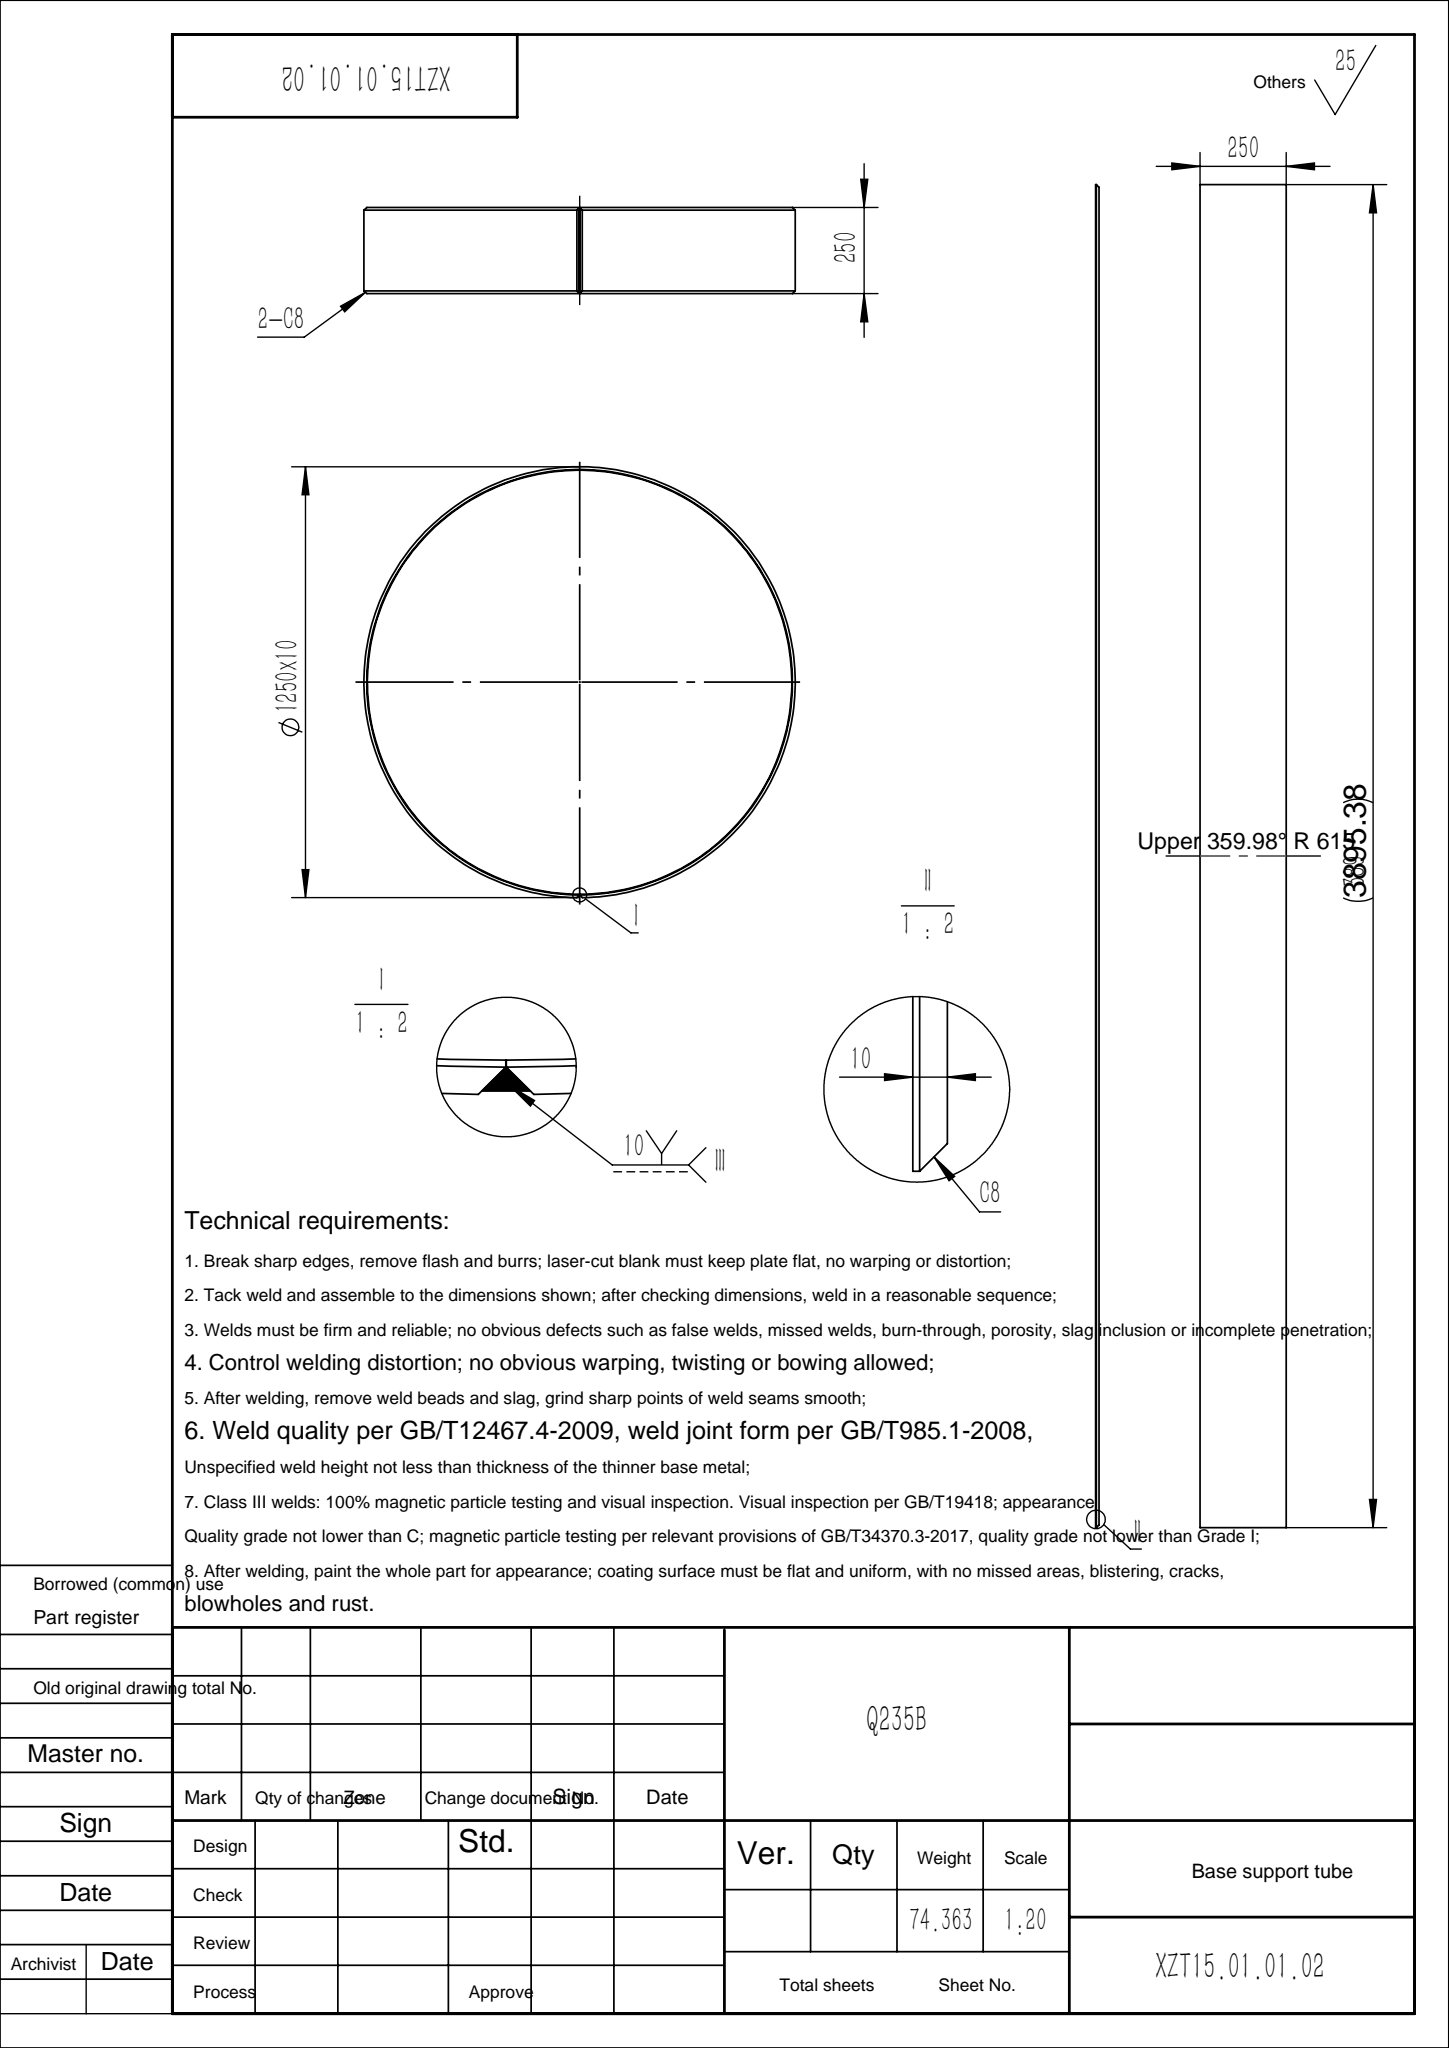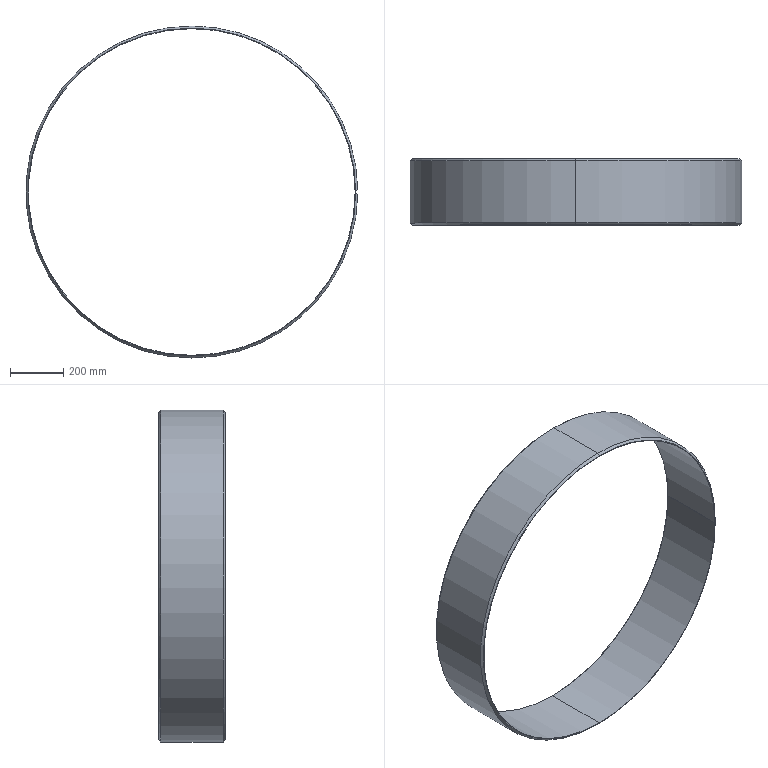Part | SolidWorks | features Chamfer 2, FlatPattern 1, SMBaseFlange 1, SheetMetal 1 | 1 solid | 18 faces | box 1250 x 250 x 1250 mm | volume 9472946 mm3 | cone 6 | cylinder 6 | plane 6 | commonest cylinder face diameters 1230 x3 1250 x3
STEP:
#1=CARTESIAN_POINT('',(0.,250.,617.));
#2=VERTEX_POINT('',#1);
#3=CARTESIAN_POINT('',(617.,250.,0.09872));
#4=VERTEX_POINT('',#3);
#5=CARTESIAN_POINT('',(0.,250.,0.));
#6=DIRECTION('',(0.,1.,0.));
#7=DIRECTION('',(0.,0.,1.));
#8=AXIS2_PLACEMENT_3D('',#5,#6,#7);
#9=CIRCLE('',#8,617.);
#10=EDGE_CURVE('',#2,#4,#9,.T.);
#11=ORIENTED_EDGE('',*,*,#10,.F.);
#12=CARTESIAN_POINT('',(0.,242.,625.));
#13=VERTEX_POINT('',#12);
#14=CARTESIAN_POINT('',(0.,250.,617.));
#15=DIRECTION('',(0.,-0.7071,0.7071));
#16=VECTOR('',#15,1000.);
#17=LINE('',#14,#16);
#18=EDGE_CURVE('',#2,#13,#17,.T.);
#19=ORIENTED_EDGE('',*,*,#18,.T.);
#20=CARTESIAN_POINT('',(624.948,242.,8.049));
#21=VERTEX_POINT('',#20);
#22=CARTESIAN_POINT('',(0.,242.,0.));
#23=DIRECTION('',(0.,-1.,0.));
#24=DIRECTION('',(0.,0.,1.));
#25=AXIS2_PLACEMENT_3D('',#22,#23,#24);
#26=CIRCLE('',#25,625.);
#27=EDGE_CURVE('',#21,#13,#26,.T.);
#28=ORIENTED_EDGE('',*,*,#27,.F.);
#29=CARTESIAN_POINT('',(624.948,242.,8.049));
#30=CARTESIAN_POINT('',(622.304,244.678,5.405));
#31=CARTESIAN_POINT('',(619.655,247.345,2.755));
#32=CARTESIAN_POINT('',(617.,250.,0.09872));
#33=B_SPLINE_CURVE_WITH_KNOTS('',3,(#29,#30,#31,#32),.UNSPECIFIED.,.F.,.F.,(4,4),(0.,0.0138),.UNSPECIFIED.);
#34=EDGE_CURVE('',#21,#4,#33,.T.);
#35=ORIENTED_EDGE('',*,*,#34,.T.);
#36=EDGE_LOOP('',(#11,#19,#28,#35));
#37=FACE_OUTER_BOUND('',#36,.T.);
#38=CARTESIAN_POINT('',(0.,250.,0.));
#39=DIRECTION('',(0.,-1.,0.));
#40=DIRECTION('',(0.,0.,-1.));
#41=AXIS2_PLACEMENT_3D('',#38,#39,#40);
#42=CONICAL_SURFACE('',#41,617.,0.7854);
#43=ADVANCED_FACE('',(#37),#42,.T.);
#44=ORIENTED_EDGE('',*,*,#18,.F.);
#45=CARTESIAN_POINT('',(0.,250.,-617.));
#46=VERTEX_POINT('',#45);
#47=CARTESIAN_POINT('',(0.,250.,0.));
#48=DIRECTION('',(0.,1.,0.));
#49=DIRECTION('',(0.,0.,1.));
#50=AXIS2_PLACEMENT_3D('',#47,#48,#49);
#51=CIRCLE('',#50,617.);
#52=EDGE_CURVE('',#46,#2,#51,.T.);
#53=ORIENTED_EDGE('',*,*,#52,.F.);
#54=CARTESIAN_POINT('',(0.,242.,-625.));
#55=VERTEX_POINT('',#54);
#56=CARTESIAN_POINT('',(0.,250.,-617.));
#57=DIRECTION('',(0.,-0.7071,-0.7071));
#58=VECTOR('',#57,1000.);
#59=LINE('',#56,#58);
#60=EDGE_CURVE('',#46,#55,#59,.T.);
#61=ORIENTED_EDGE('',*,*,#60,.T.);
#62=CARTESIAN_POINT('',(0.,242.,0.));
#63=DIRECTION('',(0.,-1.,0.));
#64=DIRECTION('',(0.,0.,1.));
#65=AXIS2_PLACEMENT_3D('',#62,#63,#64);
#66=CIRCLE('',#65,625.);
#67=EDGE_CURVE('',#13,#55,#66,.T.);
#68=ORIENTED_EDGE('',*,*,#67,.F.);
#69=EDGE_LOOP('',(#44,#53,#61,#68));
#70=FACE_OUTER_BOUND('',#69,.T.);
#71=CARTESIAN_POINT('',(0.,250.,0.));
#72=DIRECTION('',(0.,-1.,0.));
#73=DIRECTION('',(0.,0.,-1.));
#74=AXIS2_PLACEMENT_3D('',#71,#72,#73);
#75=CONICAL_SURFACE('',#74,617.,0.7854);
#76=ADVANCED_FACE('',(#70),#75,.T.);
#77=CARTESIAN_POINT('',(0.,0.,-617.));
#78=VERTEX_POINT('',#77);
#79=CARTESIAN_POINT('',(617.,0.,-0.09872));
#80=VERTEX_POINT('',#79);
#81=CARTESIAN_POINT('',(0.,0.,0.));
#82=DIRECTION('',(0.,-1.,0.));
#83=DIRECTION('',(0.,0.,1.));
#84=AXIS2_PLACEMENT_3D('',#81,#82,#83);
#85=CIRCLE('',#84,617.);
#86=EDGE_CURVE('',#78,#80,#85,.T.);
#87=ORIENTED_EDGE('',*,*,#86,.F.);
#88=CARTESIAN_POINT('',(0.,8.,-625.));
#89=VERTEX_POINT('',#88);
#90=CARTESIAN_POINT('',(0.,8.,-625.));
#91=DIRECTION('',(0.,0.7071,-0.7071));
#92=VECTOR('',#91,1000.);
#93=LINE('',#90,#92);
#94=EDGE_CURVE('',#78,#89,#93,.T.);
#95=ORIENTED_EDGE('',*,*,#94,.T.);
#96=CARTESIAN_POINT('',(624.948,8.,-8.049));
#97=VERTEX_POINT('',#96);
#98=CARTESIAN_POINT('',(0.,8.,0.));
#99=DIRECTION('',(0.,1.,0.));
#100=DIRECTION('',(0.,0.,1.));
#101=AXIS2_PLACEMENT_3D('',#98,#99,#100);
#102=CIRCLE('',#101,625.);
#103=EDGE_CURVE('',#97,#89,#102,.T.);
#104=ORIENTED_EDGE('',*,*,#103,.F.);
#105=CARTESIAN_POINT('',(624.948,8.,-8.049));
#106=CARTESIAN_POINT('',(622.304,5.322,-5.405));
#107=CARTESIAN_POINT('',(619.655,2.655,-2.755));
#108=CARTESIAN_POINT('',(617.,0.,-0.09872));
#109=B_SPLINE_CURVE_WITH_KNOTS('',3,(#105,#106,#107,#108),.UNSPECIFIED.,.F.,.F.,(4,4),(0.,0.0138),.UNSPECIFIED.);
#110=EDGE_CURVE('',#97,#80,#109,.T.);
#111=ORIENTED_EDGE('',*,*,#110,.T.);
#112=EDGE_LOOP('',(#87,#95,#104,#111));
#113=FACE_OUTER_BOUND('',#112,.T.);
#114=CARTESIAN_POINT('',(0.,8.,0.));
#115=DIRECTION('',(0.,1.,0.));
#116=DIRECTION('',(0.,0.,1.));
#117=AXIS2_PLACEMENT_3D('',#114,#115,#116);
#118=CONICAL_SURFACE('',#117,625.,0.7854);
#119=ADVANCED_FACE('',(#113),#118,.T.);
#120=ORIENTED_EDGE('',*,*,#94,.F.);
#121=CARTESIAN_POINT('',(0.,0.,617.));
#122=VERTEX_POINT('',#121);
#123=CARTESIAN_POINT('',(0.,0.,0.));
#124=DIRECTION('',(0.,-1.,0.));
#125=DIRECTION('',(0.,0.,1.));
#126=AXIS2_PLACEMENT_3D('',#123,#124,#125);
#127=CIRCLE('',#126,617.);
#128=EDGE_CURVE('',#122,#78,#127,.T.);
#129=ORIENTED_EDGE('',*,*,#128,.F.);
#130=CARTESIAN_POINT('',(0.,8.,625.));
#131=VERTEX_POINT('',#130);
#132=CARTESIAN_POINT('',(0.,8.,625.));
#133=DIRECTION('',(0.,0.7071,0.7071));
#134=VECTOR('',#133,1000.);
#135=LINE('',#132,#134);
#136=EDGE_CURVE('',#122,#131,#135,.T.);
#137=ORIENTED_EDGE('',*,*,#136,.T.);
#138=CARTESIAN_POINT('',(0.,8.,0.));
#139=DIRECTION('',(0.,1.,0.));
#140=DIRECTION('',(0.,0.,1.));
#141=AXIS2_PLACEMENT_3D('',#138,#139,#140);
#142=CIRCLE('',#141,625.);
#143=EDGE_CURVE('',#89,#131,#142,.T.);
#144=ORIENTED_EDGE('',*,*,#143,.F.);
#145=EDGE_LOOP('',(#120,#129,#137,#144));
#146=FACE_OUTER_BOUND('',#145,.T.);
#147=CARTESIAN_POINT('',(0.,8.,0.));
#148=DIRECTION('',(0.,1.,0.));
#149=DIRECTION('',(0.,0.,1.));
#150=AXIS2_PLACEMENT_3D('',#147,#148,#149);
#151=CONICAL_SURFACE('',#150,625.,0.7854);
#152=ADVANCED_FACE('',(#146),#151,.T.);
#153=CARTESIAN_POINT('',(0.,250.,-615.));
#154=VERTEX_POINT('',#153);
#155=CARTESIAN_POINT('',(0.,250.,615.));
#156=VERTEX_POINT('',#155);
#157=CARTESIAN_POINT('',(0.,250.,0.));
#158=DIRECTION('',(0.,1.,0.));
#159=DIRECTION('',(1.,0.,0.));
#160=AXIS2_PLACEMENT_3D('',#157,#158,#159);
#161=CIRCLE('',#160,615.);
#162=EDGE_CURVE('',#154,#156,#161,.T.);
#163=ORIENTED_EDGE('',*,*,#162,.T.);
#164=CARTESIAN_POINT('',(0.,0.,615.));
#165=VERTEX_POINT('',#164);
#166=CARTESIAN_POINT('',(0.,250.,615.));
#167=DIRECTION('',(0.,-1.,0.));
#168=VECTOR('',#167,1000.);
#169=LINE('',#166,#168);
#170=EDGE_CURVE('',#156,#165,#169,.T.);
#171=ORIENTED_EDGE('',*,*,#170,.T.);
#172=CARTESIAN_POINT('',(0.,0.,-615.));
#173=VERTEX_POINT('',#172);
#174=CARTESIAN_POINT('',(0.,0.,0.));
#175=DIRECTION('',(0.,1.,0.));
#176=DIRECTION('',(1.,0.,0.));
#177=AXIS2_PLACEMENT_3D('',#174,#175,#176);
#178=CIRCLE('',#177,615.);
#179=EDGE_CURVE('',#173,#165,#178,.T.);
#180=ORIENTED_EDGE('',*,*,#179,.F.);
#181=CARTESIAN_POINT('',(0.,250.,-615.));
#182=DIRECTION('',(0.,-1.,0.));
#183=VECTOR('',#182,1000.);
#184=LINE('',#181,#183);
#185=EDGE_CURVE('',#154,#173,#184,.T.);
#186=ORIENTED_EDGE('',*,*,#185,.F.);
#187=EDGE_LOOP('',(#163,#171,#180,#186));
#188=FACE_OUTER_BOUND('',#187,.T.);
#189=CARTESIAN_POINT('',(0.,250.,0.));
#190=DIRECTION('',(0.,-1.,0.));
#191=DIRECTION('',(0.,0.,-1.));
#192=AXIS2_PLACEMENT_3D('',#189,#190,#191);
#193=CYLINDRICAL_SURFACE('',#192,615.);
#194=ADVANCED_FACE('',(#188),#193,.F.);
#195=CARTESIAN_POINT('',(615.,250.,-0.0984));
#196=VERTEX_POINT('',#195);
#197=CARTESIAN_POINT('',(0.,250.,0.));
#198=DIRECTION('',(0.,1.,0.));
#199=DIRECTION('',(1.,0.,0.));
#200=AXIS2_PLACEMENT_3D('',#197,#198,#199);
#201=CIRCLE('',#200,615.);
#202=EDGE_CURVE('',#196,#154,#201,.T.);
#203=ORIENTED_EDGE('',*,*,#202,.T.);
#204=ORIENTED_EDGE('',*,*,#185,.T.);
#205=CARTESIAN_POINT('',(615.,0.,-0.0984));
#206=VERTEX_POINT('',#205);
#207=CARTESIAN_POINT('',(0.,0.,0.));
#208=DIRECTION('',(0.,1.,0.));
#209=DIRECTION('',(1.,0.,0.));
#210=AXIS2_PLACEMENT_3D('',#207,#208,#209);
#211=CIRCLE('',#210,615.);
#212=EDGE_CURVE('',#206,#173,#211,.T.);
#213=ORIENTED_EDGE('',*,*,#212,.F.);
#214=CARTESIAN_POINT('',(615.,250.,-0.0984));
#215=DIRECTION('',(0.,-1.,0.));
#216=VECTOR('',#215,1000.);
#217=LINE('',#214,#216);
#218=EDGE_CURVE('',#196,#206,#217,.T.);
#219=ORIENTED_EDGE('',*,*,#218,.F.);
#220=EDGE_LOOP('',(#203,#204,#213,#219));
#221=FACE_OUTER_BOUND('',#220,.T.);
#222=CARTESIAN_POINT('',(0.,250.,0.));
#223=DIRECTION('',(0.,-1.,0.));
#224=DIRECTION('',(0.,0.,-1.));
#225=AXIS2_PLACEMENT_3D('',#222,#223,#224);
#226=CYLINDRICAL_SURFACE('',#225,615.);
#227=ADVANCED_FACE('',(#221),#226,.F.);
#228=ORIENTED_EDGE('',*,*,#27,.T.);
#229=CARTESIAN_POINT('',(0.,250.,625.));
#230=DIRECTION('',(0.,-1.,0.));
#231=VECTOR('',#230,1000.);
#232=LINE('',#229,#231);
#233=EDGE_CURVE('',#13,#131,#232,.T.);
#234=ORIENTED_EDGE('',*,*,#233,.T.);
#235=CARTESIAN_POINT('',(624.948,8.,8.049));
#236=VERTEX_POINT('',#235);
#237=CARTESIAN_POINT('',(0.,8.,0.));
#238=DIRECTION('',(0.,1.,0.));
#239=DIRECTION('',(0.,0.,1.));
#240=AXIS2_PLACEMENT_3D('',#237,#238,#239);
#241=CIRCLE('',#240,625.);
#242=EDGE_CURVE('',#131,#236,#241,.T.);
#243=ORIENTED_EDGE('',*,*,#242,.T.);
#244=CARTESIAN_POINT('',(624.948,250.,8.049));
#245=DIRECTION('',(0.,1.,0.));
#246=VECTOR('',#245,1000.);
#247=LINE('',#244,#246);
#248=EDGE_CURVE('',#236,#21,#247,.T.);
#249=ORIENTED_EDGE('',*,*,#248,.T.);
#250=EDGE_LOOP('',(#228,#234,#243,#249));
#251=FACE_OUTER_BOUND('',#250,.T.);
#252=CARTESIAN_POINT('',(0.,250.,0.));
#253=DIRECTION('',(0.,-1.,0.));
#254=DIRECTION('',(0.,0.,-1.));
#255=AXIS2_PLACEMENT_3D('',#252,#253,#254);
#256=CYLINDRICAL_SURFACE('',#255,625.);
#257=ADVANCED_FACE('',(#251),#256,.T.);
#258=ORIENTED_EDGE('',*,*,#233,.F.);
#259=ORIENTED_EDGE('',*,*,#67,.T.);
#260=CARTESIAN_POINT('',(0.,250.,-625.));
#261=DIRECTION('',(0.,-1.,0.));
#262=VECTOR('',#261,1000.);
#263=LINE('',#260,#262);
#264=EDGE_CURVE('',#55,#89,#263,.T.);
#265=ORIENTED_EDGE('',*,*,#264,.T.);
#266=ORIENTED_EDGE('',*,*,#143,.T.);
#267=EDGE_LOOP('',(#258,#259,#265,#266));
#268=FACE_OUTER_BOUND('',#267,.T.);
#269=CARTESIAN_POINT('',(0.,250.,0.));
#270=DIRECTION('',(0.,-1.,0.));
#271=DIRECTION('',(0.,0.,-1.));
#272=AXIS2_PLACEMENT_3D('',#269,#270,#271);
#273=CYLINDRICAL_SURFACE('',#272,625.);
#274=ADVANCED_FACE('',(#268),#273,.T.);
#275=ORIENTED_EDGE('',*,*,#264,.F.);
#276=CARTESIAN_POINT('',(624.948,242.,-8.049));
#277=VERTEX_POINT('',#276);
#278=CARTESIAN_POINT('',(0.,242.,0.));
#279=DIRECTION('',(0.,-1.,0.));
#280=DIRECTION('',(0.,0.,1.));
#281=AXIS2_PLACEMENT_3D('',#278,#279,#280);
#282=CIRCLE('',#281,625.);
#283=EDGE_CURVE('',#55,#277,#282,.T.);
#284=ORIENTED_EDGE('',*,*,#283,.T.);
#285=CARTESIAN_POINT('',(624.948,250.,-8.049));
#286=DIRECTION('',(0.,-1.,0.));
#287=VECTOR('',#286,1000.);
#288=LINE('',#285,#287);
#289=EDGE_CURVE('',#277,#97,#288,.T.);
#290=ORIENTED_EDGE('',*,*,#289,.T.);
#291=ORIENTED_EDGE('',*,*,#103,.T.);
#292=EDGE_LOOP('',(#275,#284,#290,#291));
#293=FACE_OUTER_BOUND('',#292,.T.);
#294=CARTESIAN_POINT('',(0.,250.,0.));
#295=DIRECTION('',(0.,-1.,0.));
#296=DIRECTION('',(0.,0.,-1.));
#297=AXIS2_PLACEMENT_3D('',#294,#295,#296);
#298=CYLINDRICAL_SURFACE('',#297,625.);
#299=ADVANCED_FACE('',(#293),#298,.T.);
#300=CARTESIAN_POINT('',(615.,250.,0.0984));
#301=VERTEX_POINT('',#300);
#302=CARTESIAN_POINT('',(615.,250.,0.0984));
#303=DIRECTION('',(1.,0.,0.00016));
#304=VECTOR('',#303,1000.);
#305=LINE('',#302,#304);
#306=EDGE_CURVE('',#301,#4,#305,.T.);
#307=ORIENTED_EDGE('',*,*,#306,.T.);
#308=CARTESIAN_POINT('',(617.,0.,0.09872));
#309=VERTEX_POINT('',#308);
#310=CARTESIAN_POINT('',(617.,8.,0.09872));
#311=DIRECTION('',(0.,-1.,0.));
#312=VECTOR('',#311,1000.);
#313=LINE('',#310,#312);
#314=EDGE_CURVE('',#4,#309,#313,.T.);
#315=ORIENTED_EDGE('',*,*,#314,.T.);
#316=CARTESIAN_POINT('',(615.,0.,0.0984));
#317=VERTEX_POINT('',#316);
#318=CARTESIAN_POINT('',(615.,0.,0.0984));
#319=DIRECTION('',(1.,0.,0.00016));
#320=VECTOR('',#319,1000.);
#321=LINE('',#318,#320);
#322=EDGE_CURVE('',#317,#309,#321,.T.);
#323=ORIENTED_EDGE('',*,*,#322,.F.);
#324=CARTESIAN_POINT('',(615.,250.,0.0984));
#325=DIRECTION('',(0.,-1.,0.));
#326=VECTOR('',#325,1000.);
#327=LINE('',#324,#326);
#328=EDGE_CURVE('',#301,#317,#327,.T.);
#329=ORIENTED_EDGE('',*,*,#328,.F.);
#330=EDGE_LOOP('',(#307,#315,#323,#329));
#331=FACE_OUTER_BOUND('',#330,.T.);
#332=CARTESIAN_POINT('',(615.,250.,0.0984));
#333=DIRECTION('',(0.00016,0.,-1.));
#334=DIRECTION('',(-1.,0.,-0.00016));
#335=AXIS2_PLACEMENT_3D('',#332,#333,#334);
#336=PLANE('',#335);
#337=ADVANCED_FACE('',(#331),#336,.T.);
#338=ORIENTED_EDGE('',*,*,#170,.F.);
#339=CARTESIAN_POINT('',(0.,250.,0.));
#340=DIRECTION('',(0.,1.,0.));
#341=DIRECTION('',(1.,0.,0.));
#342=AXIS2_PLACEMENT_3D('',#339,#340,#341);
#343=CIRCLE('',#342,615.);
#344=EDGE_CURVE('',#156,#301,#343,.T.);
#345=ORIENTED_EDGE('',*,*,#344,.T.);
#346=ORIENTED_EDGE('',*,*,#328,.T.);
#347=CARTESIAN_POINT('',(0.,0.,0.));
#348=DIRECTION('',(0.,1.,0.));
#349=DIRECTION('',(1.,0.,0.));
#350=AXIS2_PLACEMENT_3D('',#347,#348,#349);
#351=CIRCLE('',#350,615.);
#352=EDGE_CURVE('',#165,#317,#351,.T.);
#353=ORIENTED_EDGE('',*,*,#352,.F.);
#354=EDGE_LOOP('',(#338,#345,#346,#353));
#355=FACE_OUTER_BOUND('',#354,.T.);
#356=CARTESIAN_POINT('',(0.,250.,0.));
#357=DIRECTION('',(0.,-1.,0.));
#358=DIRECTION('',(0.,0.,-1.));
#359=AXIS2_PLACEMENT_3D('',#356,#357,#358);
#360=CYLINDRICAL_SURFACE('',#359,615.);
#361=ADVANCED_FACE('',(#355),#360,.F.);
#362=CARTESIAN_POINT('',(625.,0.,-0.1));
#363=DIRECTION('',(-1.,0.,0.00016));
#364=VECTOR('',#363,1000.);
#365=LINE('',#362,#364);
#366=EDGE_CURVE('',#80,#206,#365,.T.);
#367=ORIENTED_EDGE('',*,*,#366,.F.);
#368=CARTESIAN_POINT('',(617.,250.,-0.09872));
#369=VERTEX_POINT('',#368);
#370=CARTESIAN_POINT('',(617.,242.,-0.09872));
#371=DIRECTION('',(0.,1.,0.));
#372=VECTOR('',#371,1000.);
#373=LINE('',#370,#372);
#374=EDGE_CURVE('',#80,#369,#373,.T.);
#375=ORIENTED_EDGE('',*,*,#374,.T.);
#376=CARTESIAN_POINT('',(625.,250.,-0.1));
#377=DIRECTION('',(-1.,0.,0.00016));
#378=VECTOR('',#377,1000.);
#379=LINE('',#376,#378);
#380=EDGE_CURVE('',#369,#196,#379,.T.);
#381=ORIENTED_EDGE('',*,*,#380,.T.);
#382=ORIENTED_EDGE('',*,*,#218,.T.);
#383=EDGE_LOOP('',(#367,#375,#381,#382));
#384=FACE_OUTER_BOUND('',#383,.T.);
#385=CARTESIAN_POINT('',(625.,250.,-0.1));
#386=DIRECTION('',(0.00016,0.,1.));
#387=DIRECTION('',(1.,0.,-0.00016));
#388=AXIS2_PLACEMENT_3D('',#385,#386,#387);
#389=PLANE('',#388);
#390=ADVANCED_FACE('',(#384),#389,.T.);
#391=ORIENTED_EDGE('',*,*,#380,.F.);
#392=CARTESIAN_POINT('',(0.,250.,0.));
#393=DIRECTION('',(0.,1.,0.));
#394=DIRECTION('',(0.,0.,1.));
#395=AXIS2_PLACEMENT_3D('',#392,#393,#394);
#396=CIRCLE('',#395,617.);
#397=EDGE_CURVE('',#369,#46,#396,.T.);
#398=ORIENTED_EDGE('',*,*,#397,.T.);
#399=ORIENTED_EDGE('',*,*,#52,.T.);
#400=ORIENTED_EDGE('',*,*,#10,.T.);
#401=ORIENTED_EDGE('',*,*,#306,.F.);
#402=ORIENTED_EDGE('',*,*,#344,.F.);
#403=ORIENTED_EDGE('',*,*,#162,.F.);
#404=ORIENTED_EDGE('',*,*,#202,.F.);
#405=EDGE_LOOP('',(#391,#398,#399,#400,#401,#402,#403,#404));
#406=FACE_OUTER_BOUND('',#405,.T.);
#407=CARTESIAN_POINT('',(0.,250.,0.));
#408=DIRECTION('',(0.,1.,0.));
#409=DIRECTION('',(1.,0.,0.));
#410=AXIS2_PLACEMENT_3D('',#407,#408,#409);
#411=PLANE('',#410);
#412=ADVANCED_FACE('',(#406),#411,.T.);
#413=ORIENTED_EDGE('',*,*,#322,.T.);
#414=CARTESIAN_POINT('',(0.,0.,0.));
#415=DIRECTION('',(0.,-1.,0.));
#416=DIRECTION('',(0.,0.,1.));
#417=AXIS2_PLACEMENT_3D('',#414,#415,#416);
#418=CIRCLE('',#417,617.);
#419=EDGE_CURVE('',#309,#122,#418,.T.);
#420=ORIENTED_EDGE('',*,*,#419,.T.);
#421=ORIENTED_EDGE('',*,*,#128,.T.);
#422=ORIENTED_EDGE('',*,*,#86,.T.);
#423=ORIENTED_EDGE('',*,*,#366,.T.);
#424=ORIENTED_EDGE('',*,*,#212,.T.);
#425=ORIENTED_EDGE('',*,*,#179,.T.);
#426=ORIENTED_EDGE('',*,*,#352,.T.);
#427=EDGE_LOOP('',(#413,#420,#421,#422,#423,#424,#425,#426));
#428=FACE_OUTER_BOUND('',#427,.T.);
#429=CARTESIAN_POINT('',(0.,0.,0.));
#430=DIRECTION('',(0.,1.,0.));
#431=DIRECTION('',(1.,0.,0.));
#432=AXIS2_PLACEMENT_3D('',#429,#430,#431);
#433=PLANE('',#432);
#434=ADVANCED_FACE('',(#428),#433,.F.);
#435=ORIENTED_EDGE('',*,*,#136,.F.);
#436=ORIENTED_EDGE('',*,*,#419,.F.);
#437=CARTESIAN_POINT('',(617.,0.,0.09872));
#438=CARTESIAN_POINT('',(619.655,2.655,2.755));
#439=CARTESIAN_POINT('',(622.304,5.322,5.405));
#440=CARTESIAN_POINT('',(624.948,8.,8.049));
#441=B_SPLINE_CURVE_WITH_KNOTS('',3,(#437,#438,#439,#440),.UNSPECIFIED.,.F.,.F.,(4,4),(0.,0.0138),.UNSPECIFIED.);
#442=EDGE_CURVE('',#309,#236,#441,.T.);
#443=ORIENTED_EDGE('',*,*,#442,.T.);
#444=ORIENTED_EDGE('',*,*,#242,.F.);
#445=EDGE_LOOP('',(#435,#436,#443,#444));
#446=FACE_OUTER_BOUND('',#445,.T.);
#447=CARTESIAN_POINT('',(0.,8.,0.));
#448=DIRECTION('',(0.,1.,0.));
#449=DIRECTION('',(0.,0.,1.));
#450=AXIS2_PLACEMENT_3D('',#447,#448,#449);
#451=CONICAL_SURFACE('',#450,625.,0.7854);
#452=ADVANCED_FACE('',(#446),#451,.T.);
#453=ORIENTED_EDGE('',*,*,#60,.F.);
#454=ORIENTED_EDGE('',*,*,#397,.F.);
#455=CARTESIAN_POINT('',(617.,250.,-0.09872));
#456=CARTESIAN_POINT('',(619.655,247.345,-2.755));
#457=CARTESIAN_POINT('',(622.304,244.678,-5.405));
#458=CARTESIAN_POINT('',(624.948,242.,-8.049));
#459=B_SPLINE_CURVE_WITH_KNOTS('',3,(#455,#456,#457,#458),.UNSPECIFIED.,.F.,.F.,(4,4),(0.,0.0138),.UNSPECIFIED.);
#460=EDGE_CURVE('',#369,#277,#459,.T.);
#461=ORIENTED_EDGE('',*,*,#460,.T.);
#462=ORIENTED_EDGE('',*,*,#283,.F.);
#463=EDGE_LOOP('',(#453,#454,#461,#462));
#464=FACE_OUTER_BOUND('',#463,.T.);
#465=CARTESIAN_POINT('',(0.,250.,0.));
#466=DIRECTION('',(0.,-1.,0.));
#467=DIRECTION('',(0.,0.,-1.));
#468=AXIS2_PLACEMENT_3D('',#465,#466,#467);
#469=CONICAL_SURFACE('',#468,617.,0.7854);
#470=ADVANCED_FACE('',(#464),#469,.T.);
#471=ORIENTED_EDGE('',*,*,#34,.F.);
#472=ORIENTED_EDGE('',*,*,#248,.F.);
#473=ORIENTED_EDGE('',*,*,#442,.F.);
#474=ORIENTED_EDGE('',*,*,#314,.F.);
#475=EDGE_LOOP('',(#471,#472,#473,#474));
#476=FACE_OUTER_BOUND('',#475,.T.);
#477=CARTESIAN_POINT('',(617.,250.,0.09872));
#478=DIRECTION('',(-0.7072,0.,0.707));
#479=DIRECTION('',(0.,-1.,0.));
#480=AXIS2_PLACEMENT_3D('',#477,#478,#479);
#481=PLANE('',#480);
#482=ADVANCED_FACE('',(#476),#481,.F.);
#483=ORIENTED_EDGE('',*,*,#460,.F.);
#484=ORIENTED_EDGE('',*,*,#374,.F.);
#485=ORIENTED_EDGE('',*,*,#110,.F.);
#486=ORIENTED_EDGE('',*,*,#289,.F.);
#487=EDGE_LOOP('',(#483,#484,#485,#486));
#488=FACE_OUTER_BOUND('',#487,.T.);
#489=CARTESIAN_POINT('',(624.948,250.,-8.049));
#490=DIRECTION('',(-0.7072,0.,-0.707));
#491=DIRECTION('',(0.,-1.,0.));
#492=AXIS2_PLACEMENT_3D('',#489,#490,#491);
#493=PLANE('',#492);
#494=ADVANCED_FACE('',(#488),#493,.F.);
#495=CLOSED_SHELL('',(#43,#76,#119,#152,#194,#227,#257,#274,#299,#337,#361,#390,#412,#434,#452,#470,#482,#494));
#496=MANIFOLD_SOLID_BREP('',#495);
#497=CARTESIAN_POINT('',(0.,0.,0.));
#498=DIRECTION('',(0.,0.,1.));
#499=DIRECTION('',(1.,0.,0.));
#500=AXIS2_PLACEMENT_3D('',#497,#498,#499);
#501=(LENGTH_UNIT()NAMED_UNIT(*)SI_UNIT(.MILLI.,.METRE.));
#502=UNCERTAINTY_MEASURE_WITH_UNIT(LENGTH_MEASURE(0.00001),#501,'','');
#503=(NAMED_UNIT(*)PLANE_ANGLE_UNIT()SI_UNIT($,.RADIAN.));
#504=(NAMED_UNIT(*)SI_UNIT($,.STERADIAN.)SOLID_ANGLE_UNIT());
#505=(GEOMETRIC_REPRESENTATION_CONTEXT(3)GLOBAL_UNCERTAINTY_ASSIGNED_CONTEXT((#502))GLOBAL_UNIT_ASSIGNED_CONTEXT((#501,#503,#504))REPRESENTATION_CONTEXT('',''));
#506=ADVANCED_BREP_SHAPE_REPRESENTATION('',(#496,#500),#505);